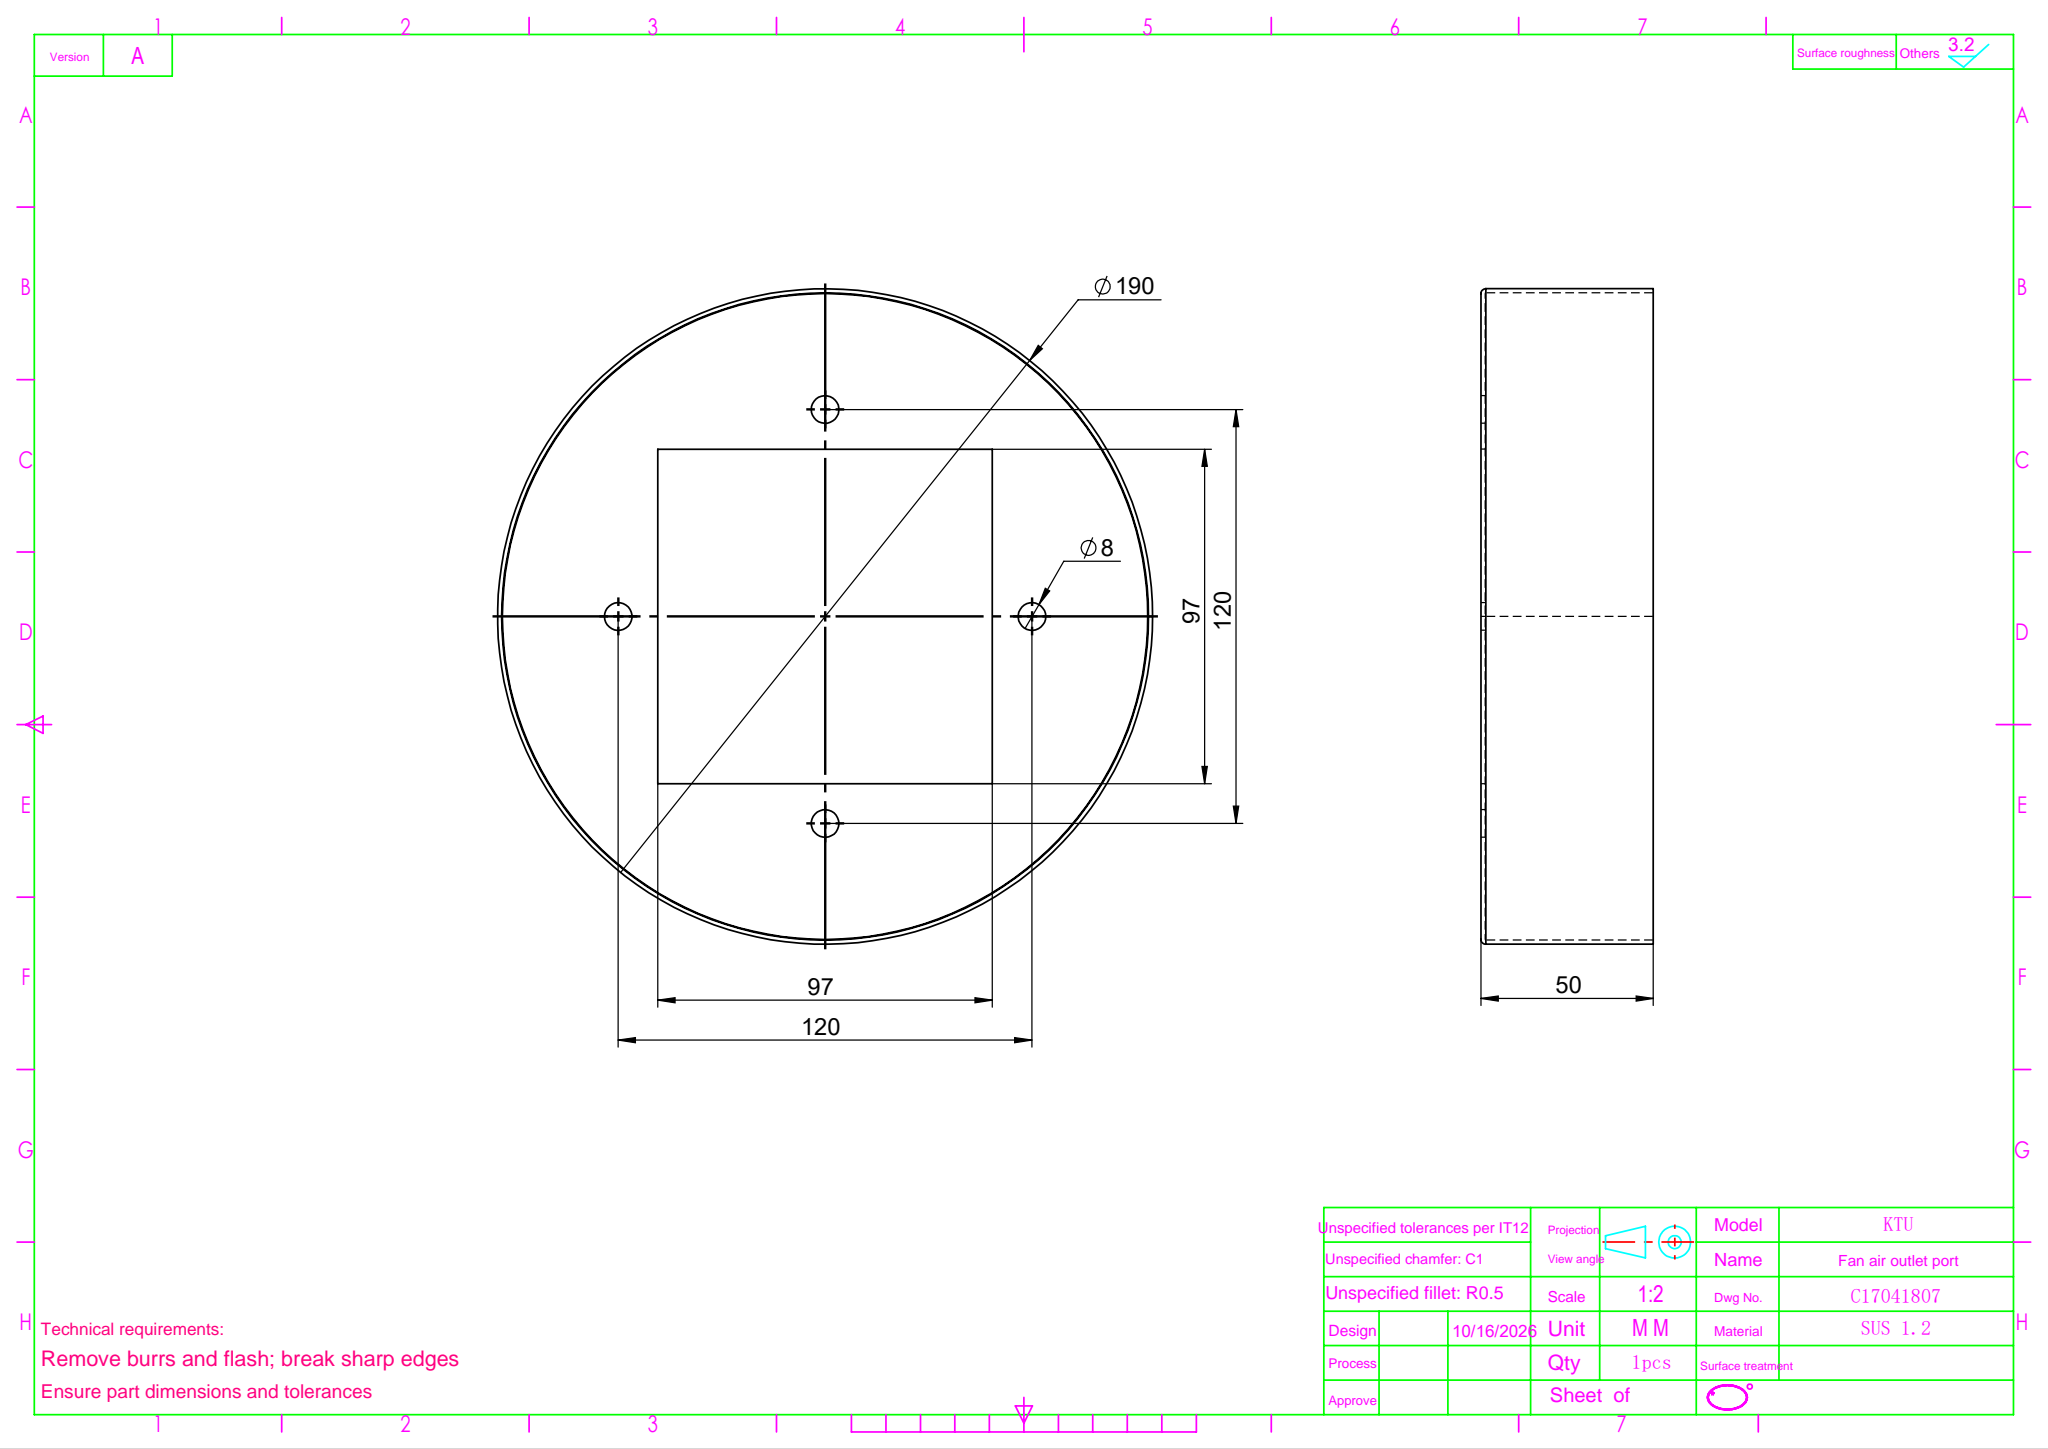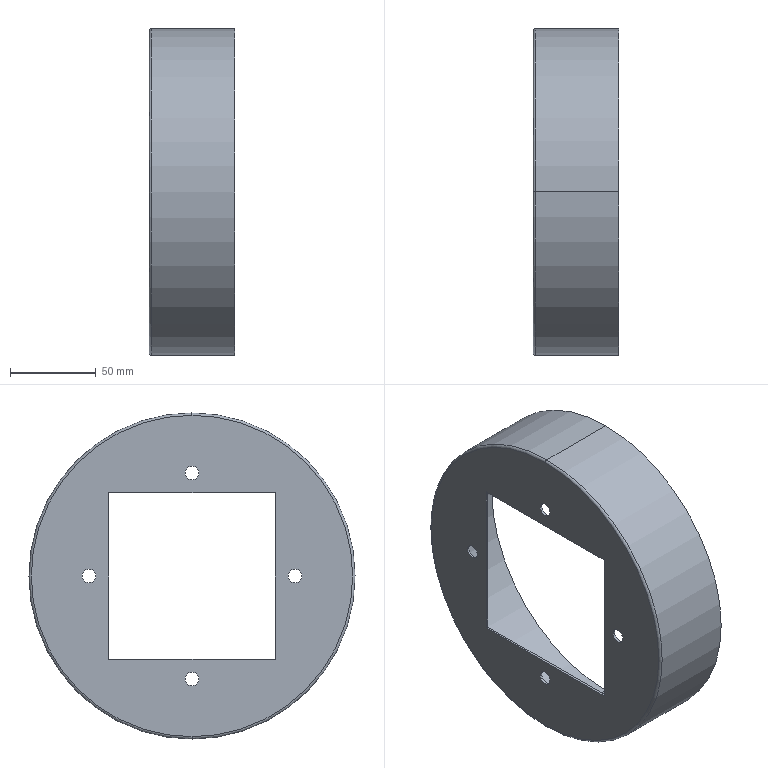Part | SolidWorks | features 3DProfileFeature 1, EdgeFlange 1, FlatPattern 1, SMBaseFlange 1, SheetMetal 1 | 1 solid | 23 faces | box 50 x 190 x 190 mm | volume 56980 mm3 | cylinder 12 | plane 7 | torus 4 | commonest cylinder face diameters 8 x8 187.6 x2 190 x2
STEP:
#1=CARTESIAN_POINT('',(-1.2,0.,-93.6));
#2=VERTEX_POINT('',#1);
#3=CARTESIAN_POINT('',(-1.2,0.,93.6));
#4=VERTEX_POINT('',#3);
#5=CARTESIAN_POINT('',(-1.2,0.,0.));
#6=DIRECTION('',(1.,0.,0.));
#7=DIRECTION('',(0.,0.,-1.));
#8=AXIS2_PLACEMENT_3D('',#5,#6,#7);
#9=CIRCLE('',#8,93.6);
#10=EDGE_CURVE('',#2,#4,#9,.T.);
#11=ORIENTED_EDGE('',*,*,#10,.T.);
#12=CARTESIAN_POINT('',(0.2,0.,95.));
#13=VERTEX_POINT('',#12);
#14=CARTESIAN_POINT('',(0.2,0.,93.6));
#15=DIRECTION('',(0.,1.,0.));
#16=DIRECTION('',(0.,0.,1.));
#17=AXIS2_PLACEMENT_3D('',#14,#15,#16);
#18=CIRCLE('',#17,1.4);
#19=EDGE_CURVE('',#4,#13,#18,.T.);
#20=ORIENTED_EDGE('',*,*,#19,.T.);
#21=CARTESIAN_POINT('',(0.2,0.,-95.));
#22=VERTEX_POINT('',#21);
#23=CARTESIAN_POINT('',(0.2,0.,0.));
#24=DIRECTION('',(1.,0.,0.));
#25=DIRECTION('',(0.,0.,-1.));
#26=AXIS2_PLACEMENT_3D('',#23,#24,#25);
#27=CIRCLE('',#26,95.);
#28=EDGE_CURVE('',#22,#13,#27,.T.);
#29=ORIENTED_EDGE('',*,*,#28,.F.);
#30=CARTESIAN_POINT('',(0.2,0.,-93.6));
#31=DIRECTION('',(0.,-1.,0.));
#32=DIRECTION('',(0.,0.,-1.));
#33=AXIS2_PLACEMENT_3D('',#30,#31,#32);
#34=CIRCLE('',#33,1.4);
#35=EDGE_CURVE('',#2,#22,#34,.T.);
#36=ORIENTED_EDGE('',*,*,#35,.F.);
#37=EDGE_LOOP('',(#11,#20,#29,#36));
#38=FACE_OUTER_BOUND('',#37,.T.);
#39=CARTESIAN_POINT('',(0.2,0.,0.));
#40=DIRECTION('',(1.,0.,0.));
#41=DIRECTION('',(0.,0.,-1.));
#42=AXIS2_PLACEMENT_3D('',#39,#40,#41);
#43=TOROIDAL_SURFACE('',#42,93.6,1.4);
#44=ADVANCED_FACE('',(#38),#43,.T.);
#45=ORIENTED_EDGE('',*,*,#28,.T.);
#46=CARTESIAN_POINT('',(48.8,0.,95.));
#47=VERTEX_POINT('',#46);
#48=CARTESIAN_POINT('',(0.,0.,95.));
#49=DIRECTION('',(1.,0.,0.));
#50=VECTOR('',#49,1000.);
#51=LINE('',#48,#50);
#52=EDGE_CURVE('',#13,#47,#51,.T.);
#53=ORIENTED_EDGE('',*,*,#52,.T.);
#54=CARTESIAN_POINT('',(48.8,0.,-95.));
#55=VERTEX_POINT('',#54);
#56=CARTESIAN_POINT('',(48.8,0.,0.));
#57=DIRECTION('',(1.,0.,0.));
#58=DIRECTION('',(0.,0.,-1.));
#59=AXIS2_PLACEMENT_3D('',#56,#57,#58);
#60=CIRCLE('',#59,95.);
#61=EDGE_CURVE('',#55,#47,#60,.T.);
#62=ORIENTED_EDGE('',*,*,#61,.F.);
#63=CARTESIAN_POINT('',(0.,0.,-95.));
#64=DIRECTION('',(1.,0.,0.));
#65=VECTOR('',#64,1000.);
#66=LINE('',#63,#65);
#67=EDGE_CURVE('',#22,#55,#66,.T.);
#68=ORIENTED_EDGE('',*,*,#67,.F.);
#69=EDGE_LOOP('',(#45,#53,#62,#68));
#70=FACE_OUTER_BOUND('',#69,.T.);
#71=CARTESIAN_POINT('',(0.,0.,0.));
#72=DIRECTION('',(1.,0.,0.));
#73=DIRECTION('',(0.,0.,-1.));
#74=AXIS2_PLACEMENT_3D('',#71,#72,#73);
#75=CYLINDRICAL_SURFACE('',#74,95.);
#76=ADVANCED_FACE('',(#70),#75,.T.);
#77=CARTESIAN_POINT('',(0.,0.,93.6));
#78=VERTEX_POINT('',#77);
#79=CARTESIAN_POINT('',(0.,0.,-93.6));
#80=VERTEX_POINT('',#79);
#81=CARTESIAN_POINT('',(0.,0.,0.));
#82=DIRECTION('',(1.,0.,0.));
#83=DIRECTION('',(0.,0.,-1.));
#84=AXIS2_PLACEMENT_3D('',#81,#82,#83);
#85=CIRCLE('',#84,93.6);
#86=EDGE_CURVE('',#78,#80,#85,.T.);
#87=ORIENTED_EDGE('',*,*,#86,.F.);
#88=CARTESIAN_POINT('',(0.2,0.,93.8));
#89=VERTEX_POINT('',#88);
#90=CARTESIAN_POINT('',(0.2,0.,93.6));
#91=DIRECTION('',(0.,1.,0.));
#92=DIRECTION('',(0.,0.,1.));
#93=AXIS2_PLACEMENT_3D('',#90,#91,#92);
#94=CIRCLE('',#93,0.2);
#95=EDGE_CURVE('',#78,#89,#94,.T.);
#96=ORIENTED_EDGE('',*,*,#95,.T.);
#97=CARTESIAN_POINT('',(0.2,0.,-93.8));
#98=VERTEX_POINT('',#97);
#99=CARTESIAN_POINT('',(0.2,0.,0.));
#100=DIRECTION('',(1.,0.,0.));
#101=DIRECTION('',(0.,0.,-1.));
#102=AXIS2_PLACEMENT_3D('',#99,#100,#101);
#103=CIRCLE('',#102,93.8);
#104=EDGE_CURVE('',#89,#98,#103,.T.);
#105=ORIENTED_EDGE('',*,*,#104,.T.);
#106=CARTESIAN_POINT('',(0.2,0.,-93.6));
#107=DIRECTION('',(0.,-1.,0.));
#108=DIRECTION('',(0.,0.,-1.));
#109=AXIS2_PLACEMENT_3D('',#106,#107,#108);
#110=CIRCLE('',#109,0.2);
#111=EDGE_CURVE('',#80,#98,#110,.T.);
#112=ORIENTED_EDGE('',*,*,#111,.F.);
#113=EDGE_LOOP('',(#87,#96,#105,#112));
#114=FACE_OUTER_BOUND('',#113,.T.);
#115=CARTESIAN_POINT('',(0.2,0.,0.));
#116=DIRECTION('',(1.,0.,0.));
#117=DIRECTION('',(0.,0.,-1.));
#118=AXIS2_PLACEMENT_3D('',#115,#116,#117);
#119=TOROIDAL_SURFACE('',#118,93.6,0.2);
#120=ADVANCED_FACE('',(#114),#119,.F.);
#121=ORIENTED_EDGE('',*,*,#104,.F.);
#122=CARTESIAN_POINT('',(48.8,0.,93.8));
#123=VERTEX_POINT('',#122);
#124=CARTESIAN_POINT('',(0.,0.,93.8));
#125=DIRECTION('',(1.,0.,0.));
#126=VECTOR('',#125,1000.);
#127=LINE('',#124,#126);
#128=EDGE_CURVE('',#89,#123,#127,.T.);
#129=ORIENTED_EDGE('',*,*,#128,.T.);
#130=CARTESIAN_POINT('',(48.8,0.,-93.8));
#131=VERTEX_POINT('',#130);
#132=CARTESIAN_POINT('',(48.8,0.,0.));
#133=DIRECTION('',(1.,0.,0.));
#134=DIRECTION('',(0.,0.,-1.));
#135=AXIS2_PLACEMENT_3D('',#132,#133,#134);
#136=CIRCLE('',#135,93.8);
#137=EDGE_CURVE('',#123,#131,#136,.T.);
#138=ORIENTED_EDGE('',*,*,#137,.T.);
#139=CARTESIAN_POINT('',(0.,0.,-93.8));
#140=DIRECTION('',(1.,0.,0.));
#141=VECTOR('',#140,1000.);
#142=LINE('',#139,#141);
#143=EDGE_CURVE('',#98,#131,#142,.T.);
#144=ORIENTED_EDGE('',*,*,#143,.F.);
#145=EDGE_LOOP('',(#121,#129,#138,#144));
#146=FACE_OUTER_BOUND('',#145,.T.);
#147=CARTESIAN_POINT('',(0.,0.,0.));
#148=DIRECTION('',(1.,0.,0.));
#149=DIRECTION('',(0.,0.,-1.));
#150=AXIS2_PLACEMENT_3D('',#147,#148,#149);
#151=CYLINDRICAL_SURFACE('',#150,93.8);
#152=ADVANCED_FACE('',(#146),#151,.F.);
#153=CARTESIAN_POINT('',(-1.2,60.,4.));
#154=VERTEX_POINT('',#153);
#155=CARTESIAN_POINT('',(-1.2,60.,-4.));
#156=VERTEX_POINT('',#155);
#157=CARTESIAN_POINT('',(-1.2,60.,0.));
#158=DIRECTION('',(1.,0.,0.));
#159=DIRECTION('',(0.,0.,1.));
#160=AXIS2_PLACEMENT_3D('',#157,#158,#159);
#161=CIRCLE('',#160,4.);
#162=EDGE_CURVE('',#154,#156,#161,.T.);
#163=ORIENTED_EDGE('',*,*,#162,.F.);
#164=CARTESIAN_POINT('',(0.,60.,4.));
#165=VERTEX_POINT('',#164);
#166=CARTESIAN_POINT('',(-1.2,60.,4.));
#167=DIRECTION('',(1.,0.,0.));
#168=VECTOR('',#167,1000.);
#169=LINE('',#166,#168);
#170=EDGE_CURVE('',#154,#165,#169,.T.);
#171=ORIENTED_EDGE('',*,*,#170,.T.);
#172=CARTESIAN_POINT('',(0.,60.,-4.));
#173=VERTEX_POINT('',#172);
#174=CARTESIAN_POINT('',(0.,60.,0.));
#175=DIRECTION('',(1.,0.,0.));
#176=DIRECTION('',(0.,0.,1.));
#177=AXIS2_PLACEMENT_3D('',#174,#175,#176);
#178=CIRCLE('',#177,4.);
#179=EDGE_CURVE('',#165,#173,#178,.T.);
#180=ORIENTED_EDGE('',*,*,#179,.T.);
#181=CARTESIAN_POINT('',(-1.2,60.,-4.));
#182=DIRECTION('',(1.,0.,0.));
#183=VECTOR('',#182,1000.);
#184=LINE('',#181,#183);
#185=EDGE_CURVE('',#156,#173,#184,.T.);
#186=ORIENTED_EDGE('',*,*,#185,.F.);
#187=EDGE_LOOP('',(#163,#171,#180,#186));
#188=FACE_OUTER_BOUND('',#187,.T.);
#189=CARTESIAN_POINT('',(-1.2,60.,0.));
#190=DIRECTION('',(1.,0.,0.));
#191=DIRECTION('',(0.,0.,-1.));
#192=AXIS2_PLACEMENT_3D('',#189,#190,#191);
#193=CYLINDRICAL_SURFACE('',#192,4.);
#194=ADVANCED_FACE('',(#188),#193,.F.);
#195=CARTESIAN_POINT('',(-1.2,-60.,4.));
#196=VERTEX_POINT('',#195);
#197=CARTESIAN_POINT('',(-1.2,-60.,-4.));
#198=VERTEX_POINT('',#197);
#199=CARTESIAN_POINT('',(-1.2,-60.,0.));
#200=DIRECTION('',(1.,0.,0.));
#201=DIRECTION('',(0.,0.,-1.));
#202=AXIS2_PLACEMENT_3D('',#199,#200,#201);
#203=CIRCLE('',#202,4.);
#204=EDGE_CURVE('',#196,#198,#203,.T.);
#205=ORIENTED_EDGE('',*,*,#204,.F.);
#206=CARTESIAN_POINT('',(0.,-60.,4.));
#207=VERTEX_POINT('',#206);
#208=CARTESIAN_POINT('',(-1.2,-60.,4.));
#209=DIRECTION('',(1.,0.,0.));
#210=VECTOR('',#209,1000.);
#211=LINE('',#208,#210);
#212=EDGE_CURVE('',#196,#207,#211,.T.);
#213=ORIENTED_EDGE('',*,*,#212,.T.);
#214=CARTESIAN_POINT('',(0.,-60.,-4.));
#215=VERTEX_POINT('',#214);
#216=CARTESIAN_POINT('',(0.,-60.,0.));
#217=DIRECTION('',(1.,0.,0.));
#218=DIRECTION('',(0.,0.,-1.));
#219=AXIS2_PLACEMENT_3D('',#216,#217,#218);
#220=CIRCLE('',#219,4.);
#221=EDGE_CURVE('',#207,#215,#220,.T.);
#222=ORIENTED_EDGE('',*,*,#221,.T.);
#223=CARTESIAN_POINT('',(-1.2,-60.,-4.));
#224=DIRECTION('',(1.,0.,0.));
#225=VECTOR('',#224,1000.);
#226=LINE('',#223,#225);
#227=EDGE_CURVE('',#198,#215,#226,.T.);
#228=ORIENTED_EDGE('',*,*,#227,.F.);
#229=EDGE_LOOP('',(#205,#213,#222,#228));
#230=FACE_OUTER_BOUND('',#229,.T.);
#231=CARTESIAN_POINT('',(-1.2,-60.,0.));
#232=DIRECTION('',(1.,0.,0.));
#233=DIRECTION('',(0.,0.,-1.));
#234=AXIS2_PLACEMENT_3D('',#231,#232,#233);
#235=CYLINDRICAL_SURFACE('',#234,4.);
#236=ADVANCED_FACE('',(#230),#235,.F.);
#237=CARTESIAN_POINT('',(-1.2,0.,64.));
#238=VERTEX_POINT('',#237);
#239=CARTESIAN_POINT('',(-1.2,0.,56.));
#240=VERTEX_POINT('',#239);
#241=CARTESIAN_POINT('',(-1.2,0.,60.));
#242=DIRECTION('',(1.,0.,0.));
#243=DIRECTION('',(0.,0.,1.));
#244=AXIS2_PLACEMENT_3D('',#241,#242,#243);
#245=CIRCLE('',#244,4.);
#246=EDGE_CURVE('',#238,#240,#245,.T.);
#247=ORIENTED_EDGE('',*,*,#246,.F.);
#248=CARTESIAN_POINT('',(0.,0.,64.));
#249=VERTEX_POINT('',#248);
#250=CARTESIAN_POINT('',(-1.2,0.,64.));
#251=DIRECTION('',(1.,0.,0.));
#252=VECTOR('',#251,1000.);
#253=LINE('',#250,#252);
#254=EDGE_CURVE('',#238,#249,#253,.T.);
#255=ORIENTED_EDGE('',*,*,#254,.T.);
#256=CARTESIAN_POINT('',(0.,0.,56.));
#257=VERTEX_POINT('',#256);
#258=CARTESIAN_POINT('',(0.,0.,60.));
#259=DIRECTION('',(1.,0.,0.));
#260=DIRECTION('',(0.,0.,1.));
#261=AXIS2_PLACEMENT_3D('',#258,#259,#260);
#262=CIRCLE('',#261,4.);
#263=EDGE_CURVE('',#249,#257,#262,.T.);
#264=ORIENTED_EDGE('',*,*,#263,.T.);
#265=CARTESIAN_POINT('',(-1.2,0.,56.));
#266=DIRECTION('',(1.,0.,0.));
#267=VECTOR('',#266,1000.);
#268=LINE('',#265,#267);
#269=EDGE_CURVE('',#240,#257,#268,.T.);
#270=ORIENTED_EDGE('',*,*,#269,.F.);
#271=EDGE_LOOP('',(#247,#255,#264,#270));
#272=FACE_OUTER_BOUND('',#271,.T.);
#273=CARTESIAN_POINT('',(-1.2,0.,60.));
#274=DIRECTION('',(1.,0.,0.));
#275=DIRECTION('',(0.,0.,-1.));
#276=AXIS2_PLACEMENT_3D('',#273,#274,#275);
#277=CYLINDRICAL_SURFACE('',#276,4.);
#278=ADVANCED_FACE('',(#272),#277,.F.);
#279=CARTESIAN_POINT('',(-1.2,0.,-56.));
#280=VERTEX_POINT('',#279);
#281=CARTESIAN_POINT('',(-1.2,0.,-64.));
#282=VERTEX_POINT('',#281);
#283=CARTESIAN_POINT('',(-1.2,0.,-60.));
#284=DIRECTION('',(1.,0.,0.));
#285=DIRECTION('',(0.,0.,-1.));
#286=AXIS2_PLACEMENT_3D('',#283,#284,#285);
#287=CIRCLE('',#286,4.);
#288=EDGE_CURVE('',#280,#282,#287,.T.);
#289=ORIENTED_EDGE('',*,*,#288,.F.);
#290=CARTESIAN_POINT('',(0.,0.,-56.));
#291=VERTEX_POINT('',#290);
#292=CARTESIAN_POINT('',(-1.2,0.,-56.));
#293=DIRECTION('',(1.,0.,0.));
#294=VECTOR('',#293,1000.);
#295=LINE('',#292,#294);
#296=EDGE_CURVE('',#280,#291,#295,.T.);
#297=ORIENTED_EDGE('',*,*,#296,.T.);
#298=CARTESIAN_POINT('',(0.,0.,-64.));
#299=VERTEX_POINT('',#298);
#300=CARTESIAN_POINT('',(0.,0.,-60.));
#301=DIRECTION('',(1.,0.,0.));
#302=DIRECTION('',(0.,0.,-1.));
#303=AXIS2_PLACEMENT_3D('',#300,#301,#302);
#304=CIRCLE('',#303,4.);
#305=EDGE_CURVE('',#291,#299,#304,.T.);
#306=ORIENTED_EDGE('',*,*,#305,.T.);
#307=CARTESIAN_POINT('',(-1.2,0.,-64.));
#308=DIRECTION('',(1.,0.,0.));
#309=VECTOR('',#308,1000.);
#310=LINE('',#307,#309);
#311=EDGE_CURVE('',#282,#299,#310,.T.);
#312=ORIENTED_EDGE('',*,*,#311,.F.);
#313=EDGE_LOOP('',(#289,#297,#306,#312));
#314=FACE_OUTER_BOUND('',#313,.T.);
#315=CARTESIAN_POINT('',(-1.2,0.,-60.));
#316=DIRECTION('',(1.,0.,0.));
#317=DIRECTION('',(0.,0.,-1.));
#318=AXIS2_PLACEMENT_3D('',#315,#316,#317);
#319=CYLINDRICAL_SURFACE('',#318,4.);
#320=ADVANCED_FACE('',(#314),#319,.F.);
#321=CARTESIAN_POINT('',(-1.2,-48.5,48.5));
#322=VERTEX_POINT('',#321);
#323=CARTESIAN_POINT('',(-1.2,-48.5,-48.5));
#324=VERTEX_POINT('',#323);
#325=CARTESIAN_POINT('',(-1.2,-48.5,48.5));
#326=DIRECTION('',(0.,0.,-1.));
#327=VECTOR('',#326,1000.);
#328=LINE('',#325,#327);
#329=EDGE_CURVE('',#322,#324,#328,.T.);
#330=ORIENTED_EDGE('',*,*,#329,.T.);
#331=CARTESIAN_POINT('',(-1.2,48.5,-48.5));
#332=VERTEX_POINT('',#331);
#333=CARTESIAN_POINT('',(-1.2,-48.5,-48.5));
#334=DIRECTION('',(0.,1.,0.));
#335=VECTOR('',#334,1000.);
#336=LINE('',#333,#335);
#337=EDGE_CURVE('',#324,#332,#336,.T.);
#338=ORIENTED_EDGE('',*,*,#337,.T.);
#339=CARTESIAN_POINT('',(-1.2,48.5,48.5));
#340=VERTEX_POINT('',#339);
#341=CARTESIAN_POINT('',(-1.2,48.5,48.5));
#342=DIRECTION('',(0.,0.,1.));
#343=VECTOR('',#342,1000.);
#344=LINE('',#341,#343);
#345=EDGE_CURVE('',#332,#340,#344,.T.);
#346=ORIENTED_EDGE('',*,*,#345,.T.);
#347=CARTESIAN_POINT('',(-1.2,-48.5,48.5));
#348=DIRECTION('',(0.,-1.,0.));
#349=VECTOR('',#348,1000.);
#350=LINE('',#347,#349);
#351=EDGE_CURVE('',#340,#322,#350,.T.);
#352=ORIENTED_EDGE('',*,*,#351,.T.);
#353=EDGE_LOOP('',(#330,#338,#346,#352));
#354=FACE_BOUND('',#353,.T.);
#355=CARTESIAN_POINT('',(-1.2,0.,-60.));
#356=DIRECTION('',(1.,0.,0.));
#357=DIRECTION('',(0.,0.,-1.));
#358=AXIS2_PLACEMENT_3D('',#355,#356,#357);
#359=CIRCLE('',#358,4.);
#360=EDGE_CURVE('',#282,#280,#359,.T.);
#361=ORIENTED_EDGE('',*,*,#360,.T.);
#362=ORIENTED_EDGE('',*,*,#288,.T.);
#363=EDGE_LOOP('',(#361,#362));
#364=FACE_BOUND('',#363,.T.);
#365=CARTESIAN_POINT('',(-1.2,0.,60.));
#366=DIRECTION('',(1.,0.,0.));
#367=DIRECTION('',(0.,0.,1.));
#368=AXIS2_PLACEMENT_3D('',#365,#366,#367);
#369=CIRCLE('',#368,4.);
#370=EDGE_CURVE('',#240,#238,#369,.T.);
#371=ORIENTED_EDGE('',*,*,#370,.T.);
#372=ORIENTED_EDGE('',*,*,#246,.T.);
#373=EDGE_LOOP('',(#371,#372));
#374=FACE_BOUND('',#373,.T.);
#375=CARTESIAN_POINT('',(-1.2,-60.,0.));
#376=DIRECTION('',(1.,0.,0.));
#377=DIRECTION('',(0.,0.,-1.));
#378=AXIS2_PLACEMENT_3D('',#375,#376,#377);
#379=CIRCLE('',#378,4.);
#380=EDGE_CURVE('',#198,#196,#379,.T.);
#381=ORIENTED_EDGE('',*,*,#380,.T.);
#382=ORIENTED_EDGE('',*,*,#204,.T.);
#383=EDGE_LOOP('',(#381,#382));
#384=FACE_BOUND('',#383,.T.);
#385=CARTESIAN_POINT('',(-1.2,60.,0.));
#386=DIRECTION('',(1.,0.,0.));
#387=DIRECTION('',(0.,0.,1.));
#388=AXIS2_PLACEMENT_3D('',#385,#386,#387);
#389=CIRCLE('',#388,4.);
#390=EDGE_CURVE('',#156,#154,#389,.T.);
#391=ORIENTED_EDGE('',*,*,#390,.T.);
#392=ORIENTED_EDGE('',*,*,#162,.T.);
#393=EDGE_LOOP('',(#391,#392));
#394=FACE_BOUND('',#393,.T.);
#395=ORIENTED_EDGE('',*,*,#10,.F.);
#396=CARTESIAN_POINT('',(-1.2,0.,0.));
#397=DIRECTION('',(1.,0.,0.));
#398=DIRECTION('',(0.,0.,-1.));
#399=AXIS2_PLACEMENT_3D('',#396,#397,#398);
#400=CIRCLE('',#399,93.6);
#401=EDGE_CURVE('',#4,#2,#400,.T.);
#402=ORIENTED_EDGE('',*,*,#401,.F.);
#403=EDGE_LOOP('',(#395,#402));
#404=FACE_OUTER_BOUND('',#403,.T.);
#405=CARTESIAN_POINT('',(-1.2,0.,0.));
#406=DIRECTION('',(1.,0.,0.));
#407=DIRECTION('',(0.,0.,-1.));
#408=AXIS2_PLACEMENT_3D('',#405,#406,#407);
#409=PLANE('',#408);
#410=ADVANCED_FACE('',(#354,#364,#374,#384,#394,#404),#409,.F.);
#411=CARTESIAN_POINT('',(0.,-48.5,-48.5));
#412=VERTEX_POINT('',#411);
#413=CARTESIAN_POINT('',(0.,48.5,-48.5));
#414=VERTEX_POINT('',#413);
#415=CARTESIAN_POINT('',(0.,-48.5,-48.5));
#416=DIRECTION('',(0.,1.,0.));
#417=VECTOR('',#416,1000.);
#418=LINE('',#415,#417);
#419=EDGE_CURVE('',#412,#414,#418,.T.);
#420=ORIENTED_EDGE('',*,*,#419,.F.);
#421=CARTESIAN_POINT('',(0.,-48.5,48.5));
#422=VERTEX_POINT('',#421);
#423=CARTESIAN_POINT('',(0.,-48.5,48.5));
#424=DIRECTION('',(0.,0.,-1.));
#425=VECTOR('',#424,1000.);
#426=LINE('',#423,#425);
#427=EDGE_CURVE('',#422,#412,#426,.T.);
#428=ORIENTED_EDGE('',*,*,#427,.F.);
#429=CARTESIAN_POINT('',(0.,48.5,48.5));
#430=VERTEX_POINT('',#429);
#431=CARTESIAN_POINT('',(0.,-48.5,48.5));
#432=DIRECTION('',(0.,-1.,0.));
#433=VECTOR('',#432,1000.);
#434=LINE('',#431,#433);
#435=EDGE_CURVE('',#430,#422,#434,.T.);
#436=ORIENTED_EDGE('',*,*,#435,.F.);
#437=CARTESIAN_POINT('',(0.,48.5,48.5));
#438=DIRECTION('',(0.,0.,1.));
#439=VECTOR('',#438,1000.);
#440=LINE('',#437,#439);
#441=EDGE_CURVE('',#414,#430,#440,.T.);
#442=ORIENTED_EDGE('',*,*,#441,.F.);
#443=EDGE_LOOP('',(#420,#428,#436,#442));
#444=FACE_BOUND('',#443,.T.);
#445=CARTESIAN_POINT('',(0.,0.,-60.));
#446=DIRECTION('',(1.,0.,0.));
#447=DIRECTION('',(0.,0.,-1.));
#448=AXIS2_PLACEMENT_3D('',#445,#446,#447);
#449=CIRCLE('',#448,4.);
#450=EDGE_CURVE('',#299,#291,#449,.T.);
#451=ORIENTED_EDGE('',*,*,#450,.F.);
#452=ORIENTED_EDGE('',*,*,#305,.F.);
#453=EDGE_LOOP('',(#451,#452));
#454=FACE_BOUND('',#453,.T.);
#455=CARTESIAN_POINT('',(0.,0.,60.));
#456=DIRECTION('',(1.,0.,0.));
#457=DIRECTION('',(0.,0.,1.));
#458=AXIS2_PLACEMENT_3D('',#455,#456,#457);
#459=CIRCLE('',#458,4.);
#460=EDGE_CURVE('',#257,#249,#459,.T.);
#461=ORIENTED_EDGE('',*,*,#460,.F.);
#462=ORIENTED_EDGE('',*,*,#263,.F.);
#463=EDGE_LOOP('',(#461,#462));
#464=FACE_BOUND('',#463,.T.);
#465=CARTESIAN_POINT('',(0.,-60.,0.));
#466=DIRECTION('',(1.,0.,0.));
#467=DIRECTION('',(0.,0.,-1.));
#468=AXIS2_PLACEMENT_3D('',#465,#466,#467);
#469=CIRCLE('',#468,4.);
#470=EDGE_CURVE('',#215,#207,#469,.T.);
#471=ORIENTED_EDGE('',*,*,#470,.F.);
#472=ORIENTED_EDGE('',*,*,#221,.F.);
#473=EDGE_LOOP('',(#471,#472));
#474=FACE_BOUND('',#473,.T.);
#475=CARTESIAN_POINT('',(0.,60.,0.));
#476=DIRECTION('',(1.,0.,0.));
#477=DIRECTION('',(0.,0.,1.));
#478=AXIS2_PLACEMENT_3D('',#475,#476,#477);
#479=CIRCLE('',#478,4.);
#480=EDGE_CURVE('',#173,#165,#479,.T.);
#481=ORIENTED_EDGE('',*,*,#480,.F.);
#482=ORIENTED_EDGE('',*,*,#179,.F.);
#483=EDGE_LOOP('',(#481,#482));
#484=FACE_BOUND('',#483,.T.);
#485=CARTESIAN_POINT('',(0.,0.,0.));
#486=DIRECTION('',(1.,0.,0.));
#487=DIRECTION('',(0.,0.,-1.));
#488=AXIS2_PLACEMENT_3D('',#485,#486,#487);
#489=CIRCLE('',#488,93.6);
#490=EDGE_CURVE('',#80,#78,#489,.T.);
#491=ORIENTED_EDGE('',*,*,#490,.T.);
#492=ORIENTED_EDGE('',*,*,#86,.T.);
#493=EDGE_LOOP('',(#491,#492));
#494=FACE_OUTER_BOUND('',#493,.T.);
#495=CARTESIAN_POINT('',(0.,0.,0.));
#496=DIRECTION('',(1.,0.,0.));
#497=DIRECTION('',(0.,0.,-1.));
#498=AXIS2_PLACEMENT_3D('',#495,#496,#497);
#499=PLANE('',#498);
#500=ADVANCED_FACE('',(#444,#454,#464,#474,#484,#494),#499,.T.);
#501=ORIENTED_EDGE('',*,*,#419,.T.);
#502=CARTESIAN_POINT('',(-1.2,48.5,-48.5));
#503=DIRECTION('',(1.,0.,0.));
#504=VECTOR('',#503,1000.);
#505=LINE('',#502,#504);
#506=EDGE_CURVE('',#332,#414,#505,.T.);
#507=ORIENTED_EDGE('',*,*,#506,.F.);
#508=ORIENTED_EDGE('',*,*,#337,.F.);
#509=CARTESIAN_POINT('',(-1.2,-48.5,-48.5));
#510=DIRECTION('',(1.,0.,0.));
#511=VECTOR('',#510,1000.);
#512=LINE('',#509,#511);
#513=EDGE_CURVE('',#324,#412,#512,.T.);
#514=ORIENTED_EDGE('',*,*,#513,.T.);
#515=EDGE_LOOP('',(#501,#507,#508,#514));
#516=FACE_OUTER_BOUND('',#515,.T.);
#517=CARTESIAN_POINT('',(-1.2,-48.5,-48.5));
#518=DIRECTION('',(0.,0.,-1.));
#519=DIRECTION('',(-1.,0.,0.));
#520=AXIS2_PLACEMENT_3D('',#517,#518,#519);
#521=PLANE('',#520);
#522=ADVANCED_FACE('',(#516),#521,.F.);
#523=ORIENTED_EDGE('',*,*,#427,.T.);
#524=ORIENTED_EDGE('',*,*,#513,.F.);
#525=ORIENTED_EDGE('',*,*,#329,.F.);
#526=CARTESIAN_POINT('',(-1.2,-48.5,48.5));
#527=DIRECTION('',(1.,0.,0.));
#528=VECTOR('',#527,1000.);
#529=LINE('',#526,#528);
#530=EDGE_CURVE('',#322,#422,#529,.T.);
#531=ORIENTED_EDGE('',*,*,#530,.T.);
#532=EDGE_LOOP('',(#523,#524,#525,#531));
#533=FACE_OUTER_BOUND('',#532,.T.);
#534=CARTESIAN_POINT('',(-1.2,-48.5,48.5));
#535=DIRECTION('',(0.,-1.,0.));
#536=DIRECTION('',(0.,0.,-1.));
#537=AXIS2_PLACEMENT_3D('',#534,#535,#536);
#538=PLANE('',#537);
#539=ADVANCED_FACE('',(#533),#538,.F.);
#540=ORIENTED_EDGE('',*,*,#435,.T.);
#541=ORIENTED_EDGE('',*,*,#530,.F.);
#542=ORIENTED_EDGE('',*,*,#351,.F.);
#543=CARTESIAN_POINT('',(-1.2,48.5,48.5));
#544=DIRECTION('',(1.,0.,0.));
#545=VECTOR('',#544,1000.);
#546=LINE('',#543,#545);
#547=EDGE_CURVE('',#340,#430,#546,.T.);
#548=ORIENTED_EDGE('',*,*,#547,.T.);
#549=EDGE_LOOP('',(#540,#541,#542,#548));
#550=FACE_OUTER_BOUND('',#549,.T.);
#551=CARTESIAN_POINT('',(-1.2,-48.5,48.5));
#552=DIRECTION('',(0.,0.,1.));
#553=DIRECTION('',(1.,0.,0.));
#554=AXIS2_PLACEMENT_3D('',#551,#552,#553);
#555=PLANE('',#554);
#556=ADVANCED_FACE('',(#550),#555,.F.);
#557=ORIENTED_EDGE('',*,*,#441,.T.);
#558=ORIENTED_EDGE('',*,*,#547,.F.);
#559=ORIENTED_EDGE('',*,*,#345,.F.);
#560=ORIENTED_EDGE('',*,*,#506,.T.);
#561=EDGE_LOOP('',(#557,#558,#559,#560));
#562=FACE_OUTER_BOUND('',#561,.T.);
#563=CARTESIAN_POINT('',(-1.2,48.5,48.5));
#564=DIRECTION('',(0.,1.,0.));
#565=DIRECTION('',(0.,0.,1.));
#566=AXIS2_PLACEMENT_3D('',#563,#564,#565);
#567=PLANE('',#566);
#568=ADVANCED_FACE('',(#562),#567,.F.);
#569=ORIENTED_EDGE('',*,*,#296,.F.);
#570=ORIENTED_EDGE('',*,*,#360,.F.);
#571=ORIENTED_EDGE('',*,*,#311,.T.);
#572=ORIENTED_EDGE('',*,*,#450,.T.);
#573=EDGE_LOOP('',(#569,#570,#571,#572));
#574=FACE_OUTER_BOUND('',#573,.T.);
#575=CARTESIAN_POINT('',(-1.2,0.,-60.));
#576=DIRECTION('',(1.,0.,0.));
#577=DIRECTION('',(0.,0.,-1.));
#578=AXIS2_PLACEMENT_3D('',#575,#576,#577);
#579=CYLINDRICAL_SURFACE('',#578,4.);
#580=ADVANCED_FACE('',(#574),#579,.F.);
#581=ORIENTED_EDGE('',*,*,#254,.F.);
#582=ORIENTED_EDGE('',*,*,#370,.F.);
#583=ORIENTED_EDGE('',*,*,#269,.T.);
#584=ORIENTED_EDGE('',*,*,#460,.T.);
#585=EDGE_LOOP('',(#581,#582,#583,#584));
#586=FACE_OUTER_BOUND('',#585,.T.);
#587=CARTESIAN_POINT('',(-1.2,0.,60.));
#588=DIRECTION('',(1.,0.,0.));
#589=DIRECTION('',(0.,0.,-1.));
#590=AXIS2_PLACEMENT_3D('',#587,#588,#589);
#591=CYLINDRICAL_SURFACE('',#590,4.);
#592=ADVANCED_FACE('',(#586),#591,.F.);
#593=ORIENTED_EDGE('',*,*,#212,.F.);
#594=ORIENTED_EDGE('',*,*,#380,.F.);
#595=ORIENTED_EDGE('',*,*,#227,.T.);
#596=ORIENTED_EDGE('',*,*,#470,.T.);
#597=EDGE_LOOP('',(#593,#594,#595,#596));
#598=FACE_OUTER_BOUND('',#597,.T.);
#599=CARTESIAN_POINT('',(-1.2,-60.,0.));
#600=DIRECTION('',(1.,0.,0.));
#601=DIRECTION('',(0.,0.,-1.));
#602=AXIS2_PLACEMENT_3D('',#599,#600,#601);
#603=CYLINDRICAL_SURFACE('',#602,4.);
#604=ADVANCED_FACE('',(#598),#603,.F.);
#605=ORIENTED_EDGE('',*,*,#170,.F.);
#606=ORIENTED_EDGE('',*,*,#390,.F.);
#607=ORIENTED_EDGE('',*,*,#185,.T.);
#608=ORIENTED_EDGE('',*,*,#480,.T.);
#609=EDGE_LOOP('',(#605,#606,#607,#608));
#610=FACE_OUTER_BOUND('',#609,.T.);
#611=CARTESIAN_POINT('',(-1.2,60.,0.));
#612=DIRECTION('',(1.,0.,0.));
#613=DIRECTION('',(0.,0.,-1.));
#614=AXIS2_PLACEMENT_3D('',#611,#612,#613);
#615=CYLINDRICAL_SURFACE('',#614,4.);
#616=ADVANCED_FACE('',(#610),#615,.F.);
#617=CARTESIAN_POINT('',(48.8,0.,0.));
#618=DIRECTION('',(1.,0.,0.));
#619=DIRECTION('',(0.,0.,-1.));
#620=AXIS2_PLACEMENT_3D('',#617,#618,#619);
#621=CIRCLE('',#620,93.8);
#622=EDGE_CURVE('',#131,#123,#621,.T.);
#623=ORIENTED_EDGE('',*,*,#622,.F.);
#624=ORIENTED_EDGE('',*,*,#137,.F.);
#625=EDGE_LOOP('',(#623,#624));
#626=FACE_BOUND('',#625,.T.);
#627=ORIENTED_EDGE('',*,*,#61,.T.);
#628=CARTESIAN_POINT('',(48.8,0.,0.));
#629=DIRECTION('',(1.,0.,0.));
#630=DIRECTION('',(0.,0.,-1.));
#631=AXIS2_PLACEMENT_3D('',#628,#629,#630);
#632=CIRCLE('',#631,95.);
#633=EDGE_CURVE('',#47,#55,#632,.T.);
#634=ORIENTED_EDGE('',*,*,#633,.T.);
#635=EDGE_LOOP('',(#627,#634));
#636=FACE_OUTER_BOUND('',#635,.T.);
#637=CARTESIAN_POINT('',(48.8,0.,0.));
#638=DIRECTION('',(-1.,0.,0.));
#639=DIRECTION('',(0.,0.,1.));
#640=AXIS2_PLACEMENT_3D('',#637,#638,#639);
#641=PLANE('',#640);
#642=ADVANCED_FACE('',(#626,#636),#641,.F.);
#643=ORIENTED_EDGE('',*,*,#128,.F.);
#644=CARTESIAN_POINT('',(0.2,0.,0.));
#645=DIRECTION('',(1.,0.,0.));
#646=DIRECTION('',(0.,0.,-1.));
#647=AXIS2_PLACEMENT_3D('',#644,#645,#646);
#648=CIRCLE('',#647,93.8);
#649=EDGE_CURVE('',#98,#89,#648,.T.);
#650=ORIENTED_EDGE('',*,*,#649,.F.);
#651=ORIENTED_EDGE('',*,*,#143,.T.);
#652=ORIENTED_EDGE('',*,*,#622,.T.);
#653=EDGE_LOOP('',(#643,#650,#651,#652));
#654=FACE_OUTER_BOUND('',#653,.T.);
#655=CARTESIAN_POINT('',(0.,0.,0.));
#656=DIRECTION('',(1.,0.,0.));
#657=DIRECTION('',(0.,0.,-1.));
#658=AXIS2_PLACEMENT_3D('',#655,#656,#657);
#659=CYLINDRICAL_SURFACE('',#658,93.8);
#660=ADVANCED_FACE('',(#654),#659,.F.);
#661=ORIENTED_EDGE('',*,*,#95,.F.);
#662=ORIENTED_EDGE('',*,*,#490,.F.);
#663=ORIENTED_EDGE('',*,*,#111,.T.);
#664=ORIENTED_EDGE('',*,*,#649,.T.);
#665=EDGE_LOOP('',(#661,#662,#663,#664));
#666=FACE_OUTER_BOUND('',#665,.T.);
#667=CARTESIAN_POINT('',(0.2,0.,0.));
#668=DIRECTION('',(1.,0.,0.));
#669=DIRECTION('',(0.,0.,-1.));
#670=AXIS2_PLACEMENT_3D('',#667,#668,#669);
#671=TOROIDAL_SURFACE('',#670,93.6,0.2);
#672=ADVANCED_FACE('',(#666),#671,.F.);
#673=ORIENTED_EDGE('',*,*,#52,.F.);
#674=CARTESIAN_POINT('',(0.2,0.,0.));
#675=DIRECTION('',(1.,0.,0.));
#676=DIRECTION('',(0.,0.,-1.));
#677=AXIS2_PLACEMENT_3D('',#674,#675,#676);
#678=CIRCLE('',#677,95.);
#679=EDGE_CURVE('',#13,#22,#678,.T.);
#680=ORIENTED_EDGE('',*,*,#679,.T.);
#681=ORIENTED_EDGE('',*,*,#67,.T.);
#682=ORIENTED_EDGE('',*,*,#633,.F.);
#683=EDGE_LOOP('',(#673,#680,#681,#682));
#684=FACE_OUTER_BOUND('',#683,.T.);
#685=CARTESIAN_POINT('',(0.,0.,0.));
#686=DIRECTION('',(1.,0.,0.));
#687=DIRECTION('',(0.,0.,-1.));
#688=AXIS2_PLACEMENT_3D('',#685,#686,#687);
#689=CYLINDRICAL_SURFACE('',#688,95.);
#690=ADVANCED_FACE('',(#684),#689,.T.);
#691=ORIENTED_EDGE('',*,*,#19,.F.);
#692=ORIENTED_EDGE('',*,*,#401,.T.);
#693=ORIENTED_EDGE('',*,*,#35,.T.);
#694=ORIENTED_EDGE('',*,*,#679,.F.);
#695=EDGE_LOOP('',(#691,#692,#693,#694));
#696=FACE_OUTER_BOUND('',#695,.T.);
#697=CARTESIAN_POINT('',(0.2,0.,0.));
#698=DIRECTION('',(1.,0.,0.));
#699=DIRECTION('',(0.,0.,-1.));
#700=AXIS2_PLACEMENT_3D('',#697,#698,#699);
#701=TOROIDAL_SURFACE('',#700,93.6,1.4);
#702=ADVANCED_FACE('',(#696),#701,.T.);
#703=CLOSED_SHELL('',(#44,#76,#120,#152,#194,#236,#278,#320,#410,#500,#522,#539,#556,#568,#580,#592,#604,#616,#642,#660,#672,#690,#702));
#704=MANIFOLD_SOLID_BREP('',#703);
#705=CARTESIAN_POINT('',(0.,0.,0.));
#706=DIRECTION('',(0.,0.,1.));
#707=DIRECTION('',(1.,0.,0.));
#708=AXIS2_PLACEMENT_3D('',#705,#706,#707);
#709=(LENGTH_UNIT()NAMED_UNIT(*)SI_UNIT(.MILLI.,.METRE.));
#710=UNCERTAINTY_MEASURE_WITH_UNIT(LENGTH_MEASURE(0.00001),#709,'','');
#711=(NAMED_UNIT(*)PLANE_ANGLE_UNIT()SI_UNIT($,.RADIAN.));
#712=(NAMED_UNIT(*)SI_UNIT($,.STERADIAN.)SOLID_ANGLE_UNIT());
#713=(GEOMETRIC_REPRESENTATION_CONTEXT(3)GLOBAL_UNCERTAINTY_ASSIGNED_CONTEXT((#710))GLOBAL_UNIT_ASSIGNED_CONTEXT((#709,#711,#712))REPRESENTATION_CONTEXT('',''));
#714=ADVANCED_BREP_SHAPE_REPRESENTATION('',(#704,#708),#713);